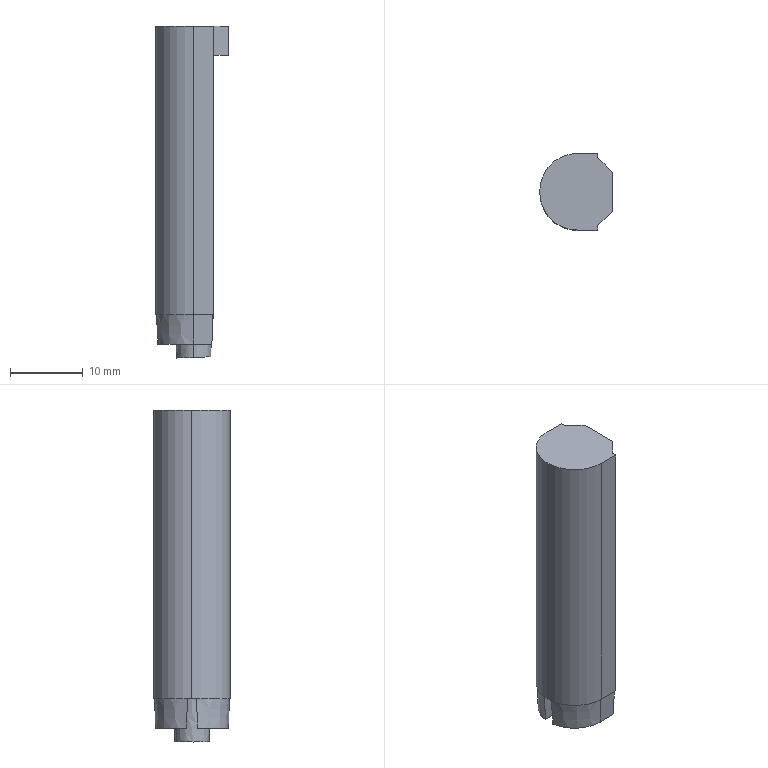Part | Creo | 1 solid | 33 faces | box 10.007 x 10.573 x 45.745 mm | volume 3201 mm3 | plane 24 | cone 4 | spline 3 | cylinder 2 | commonest cylinder face diameters 10.4 x2
STEP:
#1=CARTESIAN_POINT('',(0.,0.,0.));
#2=DIRECTION('',(0.,0.,1.));
#3=DIRECTION('',(1.,0.,0.));
#4=AXIS2_PLACEMENT_3D('',#1,#2,#3);
#5=CARTESIAN_POINT('',(40.585,-87.104,46.111));
#6=VERTEX_POINT('',#5);
#7=CARTESIAN_POINT('',(40.585,-87.104,85.91));
#8=VERTEX_POINT('',#7);
#9=CARTESIAN_POINT('',(40.585,-87.104,46.111));
#10=DIRECTION('',(0.,0.,1.));
#11=VECTOR('',#10,39.799);
#12=LINE('',#9,#11);
#13=EDGE_CURVE('',#6,#8,#12,.T.);
#14=ORIENTED_EDGE('',*,*,#13,.T.);
#15=CARTESIAN_POINT('',(43.392,-87.104,85.91));
#16=VERTEX_POINT('',#15);
#17=CARTESIAN_POINT('',(40.585,-87.104,85.91));
#18=DIRECTION('',(1.,0.,0.));
#19=VECTOR('',#18,2.807);
#20=LINE('',#17,#19);
#21=EDGE_CURVE('',#8,#16,#20,.T.);
#22=ORIENTED_EDGE('',*,*,#21,.T.);
#23=CARTESIAN_POINT('',(43.392,-87.104,46.111));
#24=VERTEX_POINT('',#23);
#25=CARTESIAN_POINT('',(43.392,-87.104,85.91));
#26=DIRECTION('',(0.,0.,-1.));
#27=VECTOR('',#26,39.799);
#28=LINE('',#25,#27);
#29=EDGE_CURVE('',#16,#24,#28,.T.);
#30=ORIENTED_EDGE('',*,*,#29,.T.);
#31=CARTESIAN_POINT('',(43.392,-87.104,46.111));
#32=DIRECTION('',(-1.,0.,0.));
#33=VECTOR('',#32,2.807);
#34=LINE('',#31,#33);
#35=EDGE_CURVE('',#24,#6,#34,.T.);
#36=ORIENTED_EDGE('',*,*,#35,.T.);
#37=EDGE_LOOP('',(#14,#22,#30,#36));
#38=FACE_OUTER_BOUND('',#37,.F.);
#39=CARTESIAN_POINT('',(39.414,-87.104,26.169));
#40=DIRECTION('',(0.,-1.,0.));
#41=DIRECTION('',(0.,0.,-1.));
#42=AXIS2_PLACEMENT_3D('',#39,#40,#41);
#43=PLANE('',#42);
#44=ADVANCED_FACE('',(#38),#43,.T.);
#45=CARTESIAN_POINT('',(35.385,-81.904,85.91));
#46=VERTEX_POINT('',#45);
#47=CARTESIAN_POINT('',(40.585,-81.904,85.91));
#48=DIRECTION('',(0.,0.,1.));
#49=DIRECTION('',(-1.,0.,0.));
#50=AXIS2_PLACEMENT_3D('',#47,#48,#49);
#51=CIRCLE('',#50,5.2);
#52=EDGE_CURVE('',#46,#8,#51,.T.);
#53=ORIENTED_EDGE('',*,*,#52,.T.);
#54=ORIENTED_EDGE('',*,*,#13,.F.);
#55=CARTESIAN_POINT('',(35.385,-81.904,46.111));
#56=VERTEX_POINT('',#55);
#57=CARTESIAN_POINT('',(40.585,-81.904,46.111));
#58=DIRECTION('',(0.,0.,-1.));
#59=DIRECTION('',(0.,-1.,0.));
#60=AXIS2_PLACEMENT_3D('',#57,#58,#59);
#61=CIRCLE('',#60,5.2);
#62=EDGE_CURVE('',#6,#56,#61,.T.);
#63=ORIENTED_EDGE('',*,*,#62,.T.);
#64=CARTESIAN_POINT('',(35.386,-81.817,46.111));
#65=VERTEX_POINT('',#64);
#66=CARTESIAN_POINT('',(40.585,-81.904,46.111));
#67=DIRECTION('',(0.,0.,-1.));
#68=DIRECTION('',(-1.,0.,0.));
#69=AXIS2_PLACEMENT_3D('',#66,#67,#68);
#70=CIRCLE('',#69,5.2);
#71=EDGE_CURVE('',#56,#65,#70,.T.);
#72=ORIENTED_EDGE('',*,*,#71,.T.);
#73=CARTESIAN_POINT('',(35.386,-81.817,85.91));
#74=VERTEX_POINT('',#73);
#75=CARTESIAN_POINT('',(35.386,-81.817,85.91));
#76=DIRECTION('',(0.,0.,-1.));
#77=VECTOR('',#76,39.799);
#78=LINE('',#75,#77);
#79=EDGE_CURVE('',#74,#65,#78,.T.);
#80=ORIENTED_EDGE('',*,*,#79,.F.);
#81=CARTESIAN_POINT('',(40.585,-81.904,85.91));
#82=DIRECTION('',(0.,0.,-1.));
#83=DIRECTION('',(-1.,0.,0.));
#84=AXIS2_PLACEMENT_3D('',#81,#82,#83);
#85=CIRCLE('',#84,5.2);
#86=EDGE_CURVE('',#46,#74,#85,.T.);
#87=ORIENTED_EDGE('',*,*,#86,.F.);
#88=EDGE_LOOP('',(#53,#54,#63,#72,#80,#87));
#89=FACE_OUTER_BOUND('',#88,.F.);
#90=CARTESIAN_POINT('',(40.585,-81.904,26.169));
#91=DIRECTION('',(0.,0.,1.));
#92=DIRECTION('',(1.,0.,0.));
#93=AXIS2_PLACEMENT_3D('',#90,#91,#92);
#94=CYLINDRICAL_SURFACE('',#93,5.2);
#95=ADVANCED_FACE('',(#89),#94,.T.);
#96=CARTESIAN_POINT('',(43.392,-86.504,85.91));
#97=VERTEX_POINT('',#96);
#98=CARTESIAN_POINT('',(43.392,-87.104,85.91));
#99=DIRECTION('',(0.,1.,0.));
#100=VECTOR('',#99,0.6);
#101=LINE('',#98,#100);
#102=EDGE_CURVE('',#16,#97,#101,.T.);
#103=ORIENTED_EDGE('',*,*,#102,.F.);
#104=ORIENTED_EDGE('',*,*,#21,.F.);
#105=ORIENTED_EDGE('',*,*,#52,.F.);
#106=ORIENTED_EDGE('',*,*,#86,.T.);
#107=CARTESIAN_POINT('',(35.385,-81.731,85.91));
#108=VERTEX_POINT('',#107);
#109=CARTESIAN_POINT('',(40.585,-81.731,85.91));
#110=DIRECTION('',(0.,0.,-1.));
#111=DIRECTION('',(-0.9999,-0.01662,0.));
#112=AXIS2_PLACEMENT_3D('',#109,#110,#111);
#113=CIRCLE('',#112,5.2);
#114=EDGE_CURVE('',#74,#108,#113,.T.);
#115=ORIENTED_EDGE('',*,*,#114,.T.);
#116=CARTESIAN_POINT('',(40.585,-76.531,85.91));
#117=VERTEX_POINT('',#116);
#118=CARTESIAN_POINT('',(40.585,-81.731,85.91));
#119=DIRECTION('',(0.,0.,1.));
#120=DIRECTION('',(0.,1.,0.));
#121=AXIS2_PLACEMENT_3D('',#118,#119,#120);
#122=CIRCLE('',#121,5.2);
#123=EDGE_CURVE('',#117,#108,#122,.T.);
#124=ORIENTED_EDGE('',*,*,#123,.F.);
#125=CARTESIAN_POINT('',(43.392,-76.531,85.91));
#126=VERTEX_POINT('',#125);
#127=CARTESIAN_POINT('',(43.392,-76.531,85.91));
#128=DIRECTION('',(-1.,0.,0.));
#129=VECTOR('',#128,2.807);
#130=LINE('',#127,#129);
#131=EDGE_CURVE('',#126,#117,#130,.T.);
#132=ORIENTED_EDGE('',*,*,#131,.F.);
#133=CARTESIAN_POINT('',(43.392,-77.131,85.91));
#134=VERTEX_POINT('',#133);
#135=CARTESIAN_POINT('',(43.392,-77.131,85.91));
#136=DIRECTION('',(0.,1.,0.));
#137=VECTOR('',#136,0.6);
#138=LINE('',#135,#137);
#139=EDGE_CURVE('',#134,#126,#138,.T.);
#140=ORIENTED_EDGE('',*,*,#139,.F.);
#141=CARTESIAN_POINT('',(45.392,-79.131,85.91));
#142=VERTEX_POINT('',#141);
#143=CARTESIAN_POINT('',(45.392,-79.131,85.91));
#144=DIRECTION('',(-0.7071,0.7071,0.));
#145=VECTOR('',#144,2.828);
#146=LINE('',#143,#145);
#147=EDGE_CURVE('',#142,#134,#146,.T.);
#148=ORIENTED_EDGE('',*,*,#147,.F.);
#149=CARTESIAN_POINT('',(45.392,-84.504,85.91));
#150=VERTEX_POINT('',#149);
#151=CARTESIAN_POINT('',(45.392,-84.504,85.91));
#152=DIRECTION('',(0.,1.,0.));
#153=VECTOR('',#152,5.373);
#154=LINE('',#151,#153);
#155=EDGE_CURVE('',#150,#142,#154,.T.);
#156=ORIENTED_EDGE('',*,*,#155,.F.);
#157=CARTESIAN_POINT('',(43.392,-86.504,85.91));
#158=DIRECTION('',(0.7071,0.7071,0.));
#159=VECTOR('',#158,2.828);
#160=LINE('',#157,#159);
#161=EDGE_CURVE('',#97,#150,#160,.T.);
#162=ORIENTED_EDGE('',*,*,#161,.F.);
#163=EDGE_LOOP('',(#103,#104,#105,#106,#115,#124,#132,#140,#148,#156,#162));
#164=FACE_OUTER_BOUND('',#163,.F.);
#165=CARTESIAN_POINT('',(62.144,-0.4125,85.91));
#166=DIRECTION('',(0.,0.,1.));
#167=DIRECTION('',(0.,1.,0.));
#168=AXIS2_PLACEMENT_3D('',#165,#166,#167);
#169=PLANE('',#168);
#170=ADVANCED_FACE('',(#164),#169,.T.);
#171=ORIENTED_EDGE('',*,*,#29,.F.);
#172=ORIENTED_EDGE('',*,*,#102,.T.);
#173=CARTESIAN_POINT('',(43.392,-86.504,81.91));
#174=VERTEX_POINT('',#173);
#175=CARTESIAN_POINT('',(43.392,-86.504,81.91));
#176=DIRECTION('',(0.,0.,1.));
#177=VECTOR('',#176,4.);
#178=LINE('',#175,#177);
#179=EDGE_CURVE('',#174,#97,#178,.T.);
#180=ORIENTED_EDGE('',*,*,#179,.F.);
#181=CARTESIAN_POINT('',(43.392,-77.131,81.91));
#182=VERTEX_POINT('',#181);
#183=CARTESIAN_POINT('',(43.392,-77.131,81.91));
#184=DIRECTION('',(0.,-1.,0.));
#185=VECTOR('',#184,9.373);
#186=LINE('',#183,#185);
#187=EDGE_CURVE('',#182,#174,#186,.T.);
#188=ORIENTED_EDGE('',*,*,#187,.F.);
#189=CARTESIAN_POINT('',(43.392,-77.131,85.91));
#190=DIRECTION('',(0.,0.,-1.));
#191=VECTOR('',#190,4.);
#192=LINE('',#189,#191);
#193=EDGE_CURVE('',#134,#182,#192,.T.);
#194=ORIENTED_EDGE('',*,*,#193,.F.);
#195=ORIENTED_EDGE('',*,*,#139,.T.);
#196=CARTESIAN_POINT('',(43.392,-76.531,46.111));
#197=VERTEX_POINT('',#196);
#198=CARTESIAN_POINT('',(43.392,-76.531,85.91));
#199=DIRECTION('',(0.,0.,-1.));
#200=VECTOR('',#199,39.799);
#201=LINE('',#198,#200);
#202=EDGE_CURVE('',#126,#197,#201,.T.);
#203=ORIENTED_EDGE('',*,*,#202,.T.);
#204=CARTESIAN_POINT('',(43.392,-76.531,46.111));
#205=DIRECTION('',(0.,-1.,0.));
#206=VECTOR('',#205,10.573);
#207=LINE('',#204,#206);
#208=EDGE_CURVE('',#197,#24,#207,.T.);
#209=ORIENTED_EDGE('',*,*,#208,.T.);
#210=EDGE_LOOP('',(#171,#172,#180,#188,#194,#195,#203,#209));
#211=FACE_OUTER_BOUND('',#210,.F.);
#212=CARTESIAN_POINT('',(43.392,-81.817,26.169));
#213=DIRECTION('',(1.,0.,0.));
#214=DIRECTION('',(0.,0.,-1.));
#215=AXIS2_PLACEMENT_3D('',#212,#213,#214);
#216=PLANE('',#215);
#217=ADVANCED_FACE('',(#211),#216,.T.);
#218=CARTESIAN_POINT('',(45.392,-84.504,81.91));
#219=VERTEX_POINT('',#218);
#220=CARTESIAN_POINT('',(45.392,-84.504,81.91));
#221=DIRECTION('',(-0.7071,-0.7071,0.));
#222=VECTOR('',#221,2.828);
#223=LINE('',#220,#222);
#224=EDGE_CURVE('',#219,#174,#223,.T.);
#225=ORIENTED_EDGE('',*,*,#224,.T.);
#226=ORIENTED_EDGE('',*,*,#179,.T.);
#227=ORIENTED_EDGE('',*,*,#161,.T.);
#228=CARTESIAN_POINT('',(45.392,-84.504,81.91));
#229=DIRECTION('',(0.,0.,1.));
#230=VECTOR('',#229,4.);
#231=LINE('',#228,#230);
#232=EDGE_CURVE('',#219,#150,#231,.T.);
#233=ORIENTED_EDGE('',*,*,#232,.F.);
#234=EDGE_LOOP('',(#225,#226,#227,#233));
#235=FACE_OUTER_BOUND('',#234,.F.);
#236=CARTESIAN_POINT('',(43.392,-86.504,81.91));
#237=DIRECTION('',(-0.7071,0.7071,0.));
#238=DIRECTION('',(0.,0.,1.));
#239=AXIS2_PLACEMENT_3D('',#236,#237,#238);
#240=PLANE('',#239);
#241=ADVANCED_FACE('',(#235),#240,.F.);
#242=CARTESIAN_POINT('',(45.392,-79.131,81.91));
#243=VERTEX_POINT('',#242);
#244=CARTESIAN_POINT('',(45.392,-79.131,81.91));
#245=DIRECTION('',(0.,-1.,0.));
#246=VECTOR('',#245,5.373);
#247=LINE('',#244,#246);
#248=EDGE_CURVE('',#243,#219,#247,.T.);
#249=ORIENTED_EDGE('',*,*,#248,.F.);
#250=CARTESIAN_POINT('',(43.392,-77.131,81.91));
#251=DIRECTION('',(0.7071,-0.7071,0.));
#252=VECTOR('',#251,2.828);
#253=LINE('',#250,#252);
#254=EDGE_CURVE('',#182,#243,#253,.T.);
#255=ORIENTED_EDGE('',*,*,#254,.F.);
#256=ORIENTED_EDGE('',*,*,#187,.T.);
#257=ORIENTED_EDGE('',*,*,#224,.F.);
#258=EDGE_LOOP('',(#249,#255,#256,#257));
#259=FACE_OUTER_BOUND('',#258,.F.);
#260=CARTESIAN_POINT('',(43.842,-81.817,81.91));
#261=DIRECTION('',(0.,0.,-1.));
#262=DIRECTION('',(-1.,0.,0.));
#263=AXIS2_PLACEMENT_3D('',#260,#261,#262);
#264=PLANE('',#263);
#265=ADVANCED_FACE('',(#259),#264,.T.);
#266=ORIENTED_EDGE('',*,*,#155,.T.);
#267=CARTESIAN_POINT('',(45.392,-79.131,85.91));
#268=DIRECTION('',(0.,0.,-1.));
#269=VECTOR('',#268,4.);
#270=LINE('',#267,#269);
#271=EDGE_CURVE('',#142,#243,#270,.T.);
#272=ORIENTED_EDGE('',*,*,#271,.T.);
#273=ORIENTED_EDGE('',*,*,#248,.T.);
#274=ORIENTED_EDGE('',*,*,#232,.T.);
#275=EDGE_LOOP('',(#266,#272,#273,#274));
#276=FACE_OUTER_BOUND('',#275,.F.);
#277=CARTESIAN_POINT('',(45.392,-81.817,81.91));
#278=DIRECTION('',(1.,0.,0.));
#279=DIRECTION('',(0.,0.,-1.));
#280=AXIS2_PLACEMENT_3D('',#277,#278,#279);
#281=PLANE('',#280);
#282=ADVANCED_FACE('',(#276),#281,.T.);
#283=ORIENTED_EDGE('',*,*,#254,.T.);
#284=ORIENTED_EDGE('',*,*,#271,.F.);
#285=ORIENTED_EDGE('',*,*,#147,.T.);
#286=ORIENTED_EDGE('',*,*,#193,.T.);
#287=EDGE_LOOP('',(#283,#284,#285,#286));
#288=FACE_OUTER_BOUND('',#287,.F.);
#289=CARTESIAN_POINT('',(45.392,-79.131,81.91));
#290=DIRECTION('',(-0.7071,-0.7071,0.));
#291=DIRECTION('',(0.,0.,1.));
#292=AXIS2_PLACEMENT_3D('',#289,#290,#291);
#293=PLANE('',#292);
#294=ADVANCED_FACE('',(#288),#293,.F.);
#295=ORIENTED_EDGE('',*,*,#202,.F.);
#296=ORIENTED_EDGE('',*,*,#131,.T.);
#297=CARTESIAN_POINT('',(40.585,-76.531,46.111));
#298=VERTEX_POINT('',#297);
#299=CARTESIAN_POINT('',(40.585,-76.531,85.91));
#300=DIRECTION('',(0.,0.,-1.));
#301=VECTOR('',#300,39.799);
#302=LINE('',#299,#301);
#303=EDGE_CURVE('',#117,#298,#302,.T.);
#304=ORIENTED_EDGE('',*,*,#303,.T.);
#305=CARTESIAN_POINT('',(40.585,-76.531,46.111));
#306=DIRECTION('',(1.,0.,0.));
#307=VECTOR('',#306,2.807);
#308=LINE('',#305,#307);
#309=EDGE_CURVE('',#298,#197,#308,.T.);
#310=ORIENTED_EDGE('',*,*,#309,.T.);
#311=EDGE_LOOP('',(#295,#296,#304,#310));
#312=FACE_OUTER_BOUND('',#311,.F.);
#313=CARTESIAN_POINT('',(39.414,-76.531,26.169));
#314=DIRECTION('',(0.,1.,0.));
#315=DIRECTION('',(0.,0.,1.));
#316=AXIS2_PLACEMENT_3D('',#313,#314,#315);
#317=PLANE('',#316);
#318=ADVANCED_FACE('',(#312),#317,.T.);
#319=ORIENTED_EDGE('',*,*,#303,.F.);
#320=ORIENTED_EDGE('',*,*,#123,.T.);
#321=ORIENTED_EDGE('',*,*,#114,.F.);
#322=ORIENTED_EDGE('',*,*,#79,.T.);
#323=CARTESIAN_POINT('',(35.385,-81.731,46.111));
#324=VERTEX_POINT('',#323);
#325=CARTESIAN_POINT('',(40.585,-81.731,46.111));
#326=DIRECTION('',(0.,0.,-1.));
#327=DIRECTION('',(-0.9999,-0.01662,0.));
#328=AXIS2_PLACEMENT_3D('',#325,#326,#327);
#329=CIRCLE('',#328,5.2);
#330=EDGE_CURVE('',#65,#324,#329,.T.);
#331=ORIENTED_EDGE('',*,*,#330,.T.);
#332=CARTESIAN_POINT('',(40.585,-81.731,46.111));
#333=DIRECTION('',(0.,0.,-1.));
#334=DIRECTION('',(-1.,0.,0.));
#335=AXIS2_PLACEMENT_3D('',#332,#333,#334);
#336=CIRCLE('',#335,5.2);
#337=EDGE_CURVE('',#324,#298,#336,.T.);
#338=ORIENTED_EDGE('',*,*,#337,.T.);
#339=EDGE_LOOP('',(#319,#320,#321,#322,#331,#338));
#340=FACE_OUTER_BOUND('',#339,.F.);
#341=CARTESIAN_POINT('',(40.585,-81.731,26.169));
#342=DIRECTION('',(0.,0.,1.));
#343=DIRECTION('',(1.,0.,0.));
#344=AXIS2_PLACEMENT_3D('',#341,#342,#343);
#345=CYLINDRICAL_SURFACE('',#344,5.2);
#346=ADVANCED_FACE('',(#340),#345,.T.);
#347=ORIENTED_EDGE('',*,*,#35,.F.);
#348=ORIENTED_EDGE('',*,*,#208,.F.);
#349=ORIENTED_EDGE('',*,*,#309,.F.);
#350=ORIENTED_EDGE('',*,*,#337,.F.);
#351=ORIENTED_EDGE('',*,*,#330,.F.);
#352=ORIENTED_EDGE('',*,*,#71,.F.);
#353=ORIENTED_EDGE('',*,*,#62,.F.);
#354=EDGE_LOOP('',(#347,#348,#349,#350,#351,#352,#353));
#355=FACE_OUTER_BOUND('',#354,.F.);
#356=CARTESIAN_POINT('',(43.268,-76.661,46.111));
#357=VERTEX_POINT('',#356);
#358=CARTESIAN_POINT('',(40.624,-76.661,46.111));
#359=VERTEX_POINT('',#358);
#360=CARTESIAN_POINT('',(43.268,-76.661,46.111));
#361=DIRECTION('',(-1.,0.,0.));
#362=VECTOR('',#361,2.644);
#363=LINE('',#360,#362);
#364=EDGE_CURVE('',#357,#359,#363,.T.);
#365=ORIENTED_EDGE('',*,*,#364,.F.);
#366=CARTESIAN_POINT('',(43.268,-78.432,46.111));
#367=VERTEX_POINT('',#366);
#368=CARTESIAN_POINT('',(43.268,-78.432,46.111));
#369=DIRECTION('',(0.,1.,0.));
#370=VECTOR('',#369,1.771);
#371=LINE('',#368,#370);
#372=EDGE_CURVE('',#367,#357,#371,.T.);
#373=ORIENTED_EDGE('',*,*,#372,.F.);
#374=CARTESIAN_POINT('',(40.624,-78.432,46.111));
#375=VERTEX_POINT('',#374);
#376=CARTESIAN_POINT('',(40.624,-78.432,46.111));
#377=DIRECTION('',(1.,0.,0.));
#378=VECTOR('',#377,2.644);
#379=LINE('',#376,#378);
#380=EDGE_CURVE('',#375,#367,#379,.T.);
#381=ORIENTED_EDGE('',*,*,#380,.F.);
#382=CARTESIAN_POINT('',(37.296,-81.195,46.111));
#383=VERTEX_POINT('',#382);
#384=CARTESIAN_POINT('',(40.624,-81.817,46.111));
#385=DIRECTION('',(0.,0.,-1.));
#386=DIRECTION('',(-0.983,0.1837,0.));
#387=AXIS2_PLACEMENT_3D('',#384,#385,#386);
#388=CIRCLE('',#387,3.386);
#389=EDGE_CURVE('',#383,#375,#388,.T.);
#390=ORIENTED_EDGE('',*,*,#389,.F.);
#391=CARTESIAN_POINT('',(35.505,-81.195,46.111));
#392=VERTEX_POINT('',#391);
#393=CARTESIAN_POINT('',(37.296,-81.195,46.111));
#394=DIRECTION('',(-1.,0.,0.));
#395=VECTOR('',#394,1.791);
#396=LINE('',#393,#395);
#397=EDGE_CURVE('',#383,#392,#396,.T.);
#398=ORIENTED_EDGE('',*,*,#397,.T.);
#399=CARTESIAN_POINT('',(40.624,-81.817,46.111));
#400=DIRECTION('',(0.,0.,1.));
#401=DIRECTION('',(0.,1.,0.));
#402=AXIS2_PLACEMENT_3D('',#399,#400,#401);
#403=CIRCLE('',#402,5.157);
#404=EDGE_CURVE('',#359,#392,#403,.T.);
#405=ORIENTED_EDGE('',*,*,#404,.F.);
#406=EDGE_LOOP('',(#365,#373,#381,#390,#398,#405));
#407=FACE_BOUND('',#406,.F.);
#408=CARTESIAN_POINT('',(40.625,-84.381,46.111));
#409=VERTEX_POINT('',#408);
#410=CARTESIAN_POINT('',(40.626,-79.254,46.111));
#411=VERTEX_POINT('',#410);
#412=CARTESIAN_POINT('',(40.625,-84.381,46.111));
#413=CARTESIAN_POINT('',(40.443,-84.382,46.111));
#414=CARTESIAN_POINT('',(40.091,-84.345,46.111));
#415=CARTESIAN_POINT('',(39.576,-84.179,46.111));
#416=CARTESIAN_POINT('',(39.107,-83.909,46.111));
#417=CARTESIAN_POINT('',(38.709,-83.552,46.111));
#418=CARTESIAN_POINT('',(38.389,-83.115,46.111));
#419=CARTESIAN_POINT('',(38.168,-82.62,46.111));
#420=CARTESIAN_POINT('',(38.055,-82.091,46.111));
#421=CARTESIAN_POINT('',(38.054,-81.551,46.111));
#422=CARTESIAN_POINT('',(38.166,-81.023,46.111));
#423=CARTESIAN_POINT('',(38.384,-80.529,46.111));
#424=CARTESIAN_POINT('',(38.702,-80.091,46.111));
#425=CARTESIAN_POINT('',(39.1,-79.731,46.111));
#426=CARTESIAN_POINT('',(39.57,-79.458,46.111));
#427=CARTESIAN_POINT('',(40.089,-79.291,46.111));
#428=CARTESIAN_POINT('',(40.442,-79.253,46.111));
#429=CARTESIAN_POINT('',(40.626,-79.254,46.111));
#430=B_SPLINE_CURVE_WITH_KNOTS('',3,(#412,#413,#414,#415,#416,#417,#418,#419,#420,#421,#422,#423,#424,#425,#426,#427,#428,#429),.UNSPECIFIED.,.F.,.F.,(4,1,1,1,1,1,1,1,1,1,1,1,1,1,1,4),(0.,0.06667,0.1333,0.2,0.2667,0.3333,0.4,0.4667,0.5333,0.6,0.6667,0.7333,0.8,0.8667,0.9333,1.),.UNSPECIFIED.);
#431=EDGE_CURVE('',#409,#411,#430,.T.);
#432=ORIENTED_EDGE('',*,*,#431,.T.);
#433=CARTESIAN_POINT('',(41.074,-79.294,46.111));
#434=VERTEX_POINT('',#433);
#435=CARTESIAN_POINT('',(40.626,-79.254,46.111));
#436=CARTESIAN_POINT('',(40.674,-79.254,46.111));
#437=CARTESIAN_POINT('',(40.776,-79.257,46.111));
#438=CARTESIAN_POINT('',(40.926,-79.27,46.111));
#439=CARTESIAN_POINT('',(41.024,-79.285,46.111));
#440=B_SPLINE_CURVE_WITH_KNOTS('',3,(#435,#436,#437,#438,#439,#433),.UNSPECIFIED.,.F.,.F.,(4,1,1,4),(0.,0.3333,0.6667,1.),.UNSPECIFIED.);
#441=EDGE_CURVE('',#411,#434,#440,.T.);
#442=ORIENTED_EDGE('',*,*,#441,.T.);
#443=CARTESIAN_POINT('',(43.303,-79.295,46.111));
#444=VERTEX_POINT('',#443);
#445=CARTESIAN_POINT('',(43.303,-79.295,46.111));
#446=DIRECTION('',(-1.,0.0001161,-0.000004118));
#447=VECTOR('',#446,2.23);
#448=LINE('',#445,#447);
#449=EDGE_CURVE('',#444,#434,#448,.T.);
#450=ORIENTED_EDGE('',*,*,#449,.F.);
#451=CARTESIAN_POINT('',(43.303,-84.34,46.111));
#452=VERTEX_POINT('',#451);
#453=CARTESIAN_POINT('',(43.303,-84.34,46.111));
#454=DIRECTION('',(0.,1.,0.));
#455=VECTOR('',#454,5.046);
#456=LINE('',#453,#455);
#457=EDGE_CURVE('',#452,#444,#456,.T.);
#458=ORIENTED_EDGE('',*,*,#457,.F.);
#459=CARTESIAN_POINT('',(41.071,-84.341,46.111));
#460=VERTEX_POINT('',#459);
#461=CARTESIAN_POINT('',(41.071,-84.341,46.111));
#462=DIRECTION('',(1.,0.0002341,0.000008303));
#463=VECTOR('',#462,2.232);
#464=LINE('',#461,#463);
#465=EDGE_CURVE('',#460,#452,#464,.T.);
#466=ORIENTED_EDGE('',*,*,#465,.F.);
#467=CARTESIAN_POINT('',(40.625,-84.381,46.111));
#468=CARTESIAN_POINT('',(40.674,-84.381,46.111));
#469=CARTESIAN_POINT('',(40.774,-84.378,46.111));
#470=CARTESIAN_POINT('',(40.923,-84.364,46.111));
#471=CARTESIAN_POINT('',(41.022,-84.35,46.111));
#472=CARTESIAN_POINT('',(41.071,-84.341,46.111));
#473=B_SPLINE_CURVE_WITH_KNOTS('',3,(#467,#468,#469,#470,#471,#472),.UNSPECIFIED.,.F.,.F.,(4,1,1,4),(0.,0.3333,0.6667,1.),.UNSPECIFIED.);
#474=EDGE_CURVE('',#409,#460,#473,.T.);
#475=ORIENTED_EDGE('',*,*,#474,.F.);
#476=EDGE_LOOP('',(#432,#442,#450,#458,#466,#475));
#477=FACE_BOUND('',#476,.F.);
#478=CARTESIAN_POINT('',(43.268,-85.203,46.111));
#479=VERTEX_POINT('',#478);
#480=CARTESIAN_POINT('',(40.624,-85.203,46.111));
#481=VERTEX_POINT('',#480);
#482=CARTESIAN_POINT('',(43.268,-85.203,46.111));
#483=DIRECTION('',(-1.,0.,0.));
#484=VECTOR('',#483,2.644);
#485=LINE('',#482,#484);
#486=EDGE_CURVE('',#479,#481,#485,.T.);
#487=ORIENTED_EDGE('',*,*,#486,.F.);
#488=CARTESIAN_POINT('',(43.268,-86.974,46.111));
#489=VERTEX_POINT('',#488);
#490=CARTESIAN_POINT('',(43.268,-86.974,46.111));
#491=DIRECTION('',(0.,1.,0.));
#492=VECTOR('',#491,1.771);
#493=LINE('',#490,#492);
#494=EDGE_CURVE('',#489,#479,#493,.T.);
#495=ORIENTED_EDGE('',*,*,#494,.F.);
#496=CARTESIAN_POINT('',(40.624,-86.974,46.111));
#497=VERTEX_POINT('',#496);
#498=CARTESIAN_POINT('',(40.624,-86.974,46.111));
#499=DIRECTION('',(1.,0.,0.));
#500=VECTOR('',#499,2.644);
#501=LINE('',#498,#500);
#502=EDGE_CURVE('',#497,#489,#501,.T.);
#503=ORIENTED_EDGE('',*,*,#502,.F.);
#504=CARTESIAN_POINT('',(35.505,-82.44,46.111));
#505=VERTEX_POINT('',#504);
#506=CARTESIAN_POINT('',(40.624,-81.817,46.111));
#507=DIRECTION('',(0.,0.,1.));
#508=DIRECTION('',(-0.9927,-0.1206,0.));
#509=AXIS2_PLACEMENT_3D('',#506,#507,#508);
#510=CIRCLE('',#509,5.157);
#511=EDGE_CURVE('',#505,#497,#510,.T.);
#512=ORIENTED_EDGE('',*,*,#511,.F.);
#513=CARTESIAN_POINT('',(37.296,-82.44,46.111));
#514=VERTEX_POINT('',#513);
#515=CARTESIAN_POINT('',(35.505,-82.44,46.111));
#516=DIRECTION('',(1.,0.,0.));
#517=VECTOR('',#516,1.791);
#518=LINE('',#515,#517);
#519=EDGE_CURVE('',#505,#514,#518,.T.);
#520=ORIENTED_EDGE('',*,*,#519,.T.);
#521=CARTESIAN_POINT('',(40.624,-81.817,46.111));
#522=DIRECTION('',(0.,0.,-1.));
#523=DIRECTION('',(0.,-1.,0.));
#524=AXIS2_PLACEMENT_3D('',#521,#522,#523);
#525=CIRCLE('',#524,3.386);
#526=EDGE_CURVE('',#481,#514,#525,.T.);
#527=ORIENTED_EDGE('',*,*,#526,.F.);
#528=EDGE_LOOP('',(#487,#495,#503,#512,#520,#527));
#529=FACE_BOUND('',#528,.F.);
#530=CARTESIAN_POINT('',(17.66,-88.35,46.111));
#531=DIRECTION('',(0.,0.,1.));
#532=DIRECTION('',(-1.,0.,0.));
#533=AXIS2_PLACEMENT_3D('',#530,#531,#532);
#534=PLANE('',#533);
#535=ADVANCED_FACE('',(#355,#407,#477,#529),#534,.F.);
#536=CARTESIAN_POINT('',(43.128,-76.801,42.091));
#537=VERTEX_POINT('',#536);
#538=CARTESIAN_POINT('',(43.268,-76.661,46.111));
#539=DIRECTION('',(-0.03488,-0.03488,-0.9988));
#540=VECTOR('',#539,4.025);
#541=LINE('',#538,#540);
#542=EDGE_CURVE('',#357,#537,#541,.T.);
#543=ORIENTED_EDGE('',*,*,#542,.F.);
#544=ORIENTED_EDGE('',*,*,#364,.T.);
#545=CARTESIAN_POINT('',(40.624,-76.801,42.091));
#546=VERTEX_POINT('',#545);
#547=CARTESIAN_POINT('',(40.624,-76.661,46.111));
#548=DIRECTION('',(0.,-0.0349,-0.9994));
#549=VECTOR('',#548,4.022);
#550=LINE('',#547,#549);
#551=EDGE_CURVE('',#359,#546,#550,.T.);
#552=ORIENTED_EDGE('',*,*,#551,.T.);
#553=CARTESIAN_POINT('',(43.128,-76.801,42.091));
#554=DIRECTION('',(-1.,0.,0.));
#555=VECTOR('',#554,2.504);
#556=LINE('',#553,#555);
#557=EDGE_CURVE('',#537,#546,#556,.T.);
#558=ORIENTED_EDGE('',*,*,#557,.F.);
#559=EDGE_LOOP('',(#543,#544,#552,#558));
#560=FACE_OUTER_BOUND('',#559,.F.);
#561=CARTESIAN_POINT('',(43.137,-76.801,42.091));
#562=DIRECTION('',(0.,0.9994,-0.0349));
#563=DIRECTION('',(0.,0.0349,0.9994));
#564=AXIS2_PLACEMENT_3D('',#561,#562,#563);
#565=PLANE('',#564);
#566=ADVANCED_FACE('',(#560),#565,.T.);
#567=CARTESIAN_POINT('',(43.128,-78.291,42.091));
#568=VERTEX_POINT('',#567);
#569=CARTESIAN_POINT('',(43.268,-78.432,46.111));
#570=DIRECTION('',(-0.03488,0.03488,-0.9988));
#571=VECTOR('',#570,4.025);
#572=LINE('',#569,#571);
#573=EDGE_CURVE('',#367,#568,#572,.T.);
#574=ORIENTED_EDGE('',*,*,#573,.F.);
#575=ORIENTED_EDGE('',*,*,#372,.T.);
#576=ORIENTED_EDGE('',*,*,#542,.T.);
#577=CARTESIAN_POINT('',(43.128,-76.801,42.091));
#578=DIRECTION('',(0.,-1.,0.));
#579=VECTOR('',#578,1.49);
#580=LINE('',#577,#579);
#581=EDGE_CURVE('',#537,#568,#580,.T.);
#582=ORIENTED_EDGE('',*,*,#581,.T.);
#583=EDGE_LOOP('',(#574,#575,#576,#582));
#584=FACE_OUTER_BOUND('',#583,.F.);
#585=CARTESIAN_POINT('',(43.128,-88.35,42.091));
#586=DIRECTION('',(0.9994,0.,-0.0349));
#587=DIRECTION('',(-0.0349,0.,-0.9994));
#588=AXIS2_PLACEMENT_3D('',#585,#586,#587);
#589=PLANE('',#588);
#590=ADVANCED_FACE('',(#584),#589,.T.);
#591=ORIENTED_EDGE('',*,*,#573,.T.);
#592=CARTESIAN_POINT('',(40.624,-78.291,42.091));
#593=VERTEX_POINT('',#592);
#594=CARTESIAN_POINT('',(40.624,-78.291,42.091));
#595=DIRECTION('',(1.,0.,0.));
#596=VECTOR('',#595,2.504);
#597=LINE('',#594,#596);
#598=EDGE_CURVE('',#593,#568,#597,.T.);
#599=ORIENTED_EDGE('',*,*,#598,.F.);
#600=CARTESIAN_POINT('',(40.624,-78.291,42.091));
#601=DIRECTION('',(0.,-0.0349,0.9994));
#602=VECTOR('',#601,4.022);
#603=LINE('',#600,#602);
#604=EDGE_CURVE('',#593,#375,#603,.T.);
#605=ORIENTED_EDGE('',*,*,#604,.T.);
#606=ORIENTED_EDGE('',*,*,#380,.T.);
#607=EDGE_LOOP('',(#591,#599,#605,#606));
#608=FACE_OUTER_BOUND('',#607,.F.);
#609=CARTESIAN_POINT('',(40.624,-78.291,42.091));
#610=DIRECTION('',(0.,-0.9994,-0.0349));
#611=DIRECTION('',(0.,0.0349,-0.9994));
#612=AXIS2_PLACEMENT_3D('',#609,#610,#611);
#613=PLANE('',#612);
#614=ADVANCED_FACE('',(#608),#613,.T.);
#615=ORIENTED_EDGE('',*,*,#581,.F.);
#616=ORIENTED_EDGE('',*,*,#557,.T.);
#617=CARTESIAN_POINT('',(35.666,-81.055,42.091));
#618=VERTEX_POINT('',#617);
#619=CARTESIAN_POINT('',(40.624,-81.817,42.091));
#620=DIRECTION('',(0.,0.,-1.));
#621=DIRECTION('',(-0.9884,0.152,0.));
#622=AXIS2_PLACEMENT_3D('',#619,#620,#621);
#623=CIRCLE('',#622,5.016);
#624=EDGE_CURVE('',#618,#546,#623,.T.);
#625=ORIENTED_EDGE('',*,*,#624,.F.);
#626=CARTESIAN_POINT('',(37.181,-81.055,42.091));
#627=VERTEX_POINT('',#626);
#628=CARTESIAN_POINT('',(37.181,-81.055,42.091));
#629=DIRECTION('',(-1.,0.,0.));
#630=VECTOR('',#629,1.515);
#631=LINE('',#628,#630);
#632=EDGE_CURVE('',#627,#618,#631,.T.);
#633=ORIENTED_EDGE('',*,*,#632,.F.);
#634=CARTESIAN_POINT('',(40.624,-81.817,42.091));
#635=DIRECTION('',(0.,0.,1.));
#636=DIRECTION('',(0.,1.,0.));
#637=AXIS2_PLACEMENT_3D('',#634,#635,#636);
#638=CIRCLE('',#637,3.526);
#639=EDGE_CURVE('',#593,#627,#638,.T.);
#640=ORIENTED_EDGE('',*,*,#639,.F.);
#641=ORIENTED_EDGE('',*,*,#598,.T.);
#642=EDGE_LOOP('',(#615,#616,#625,#633,#640,#641));
#643=FACE_OUTER_BOUND('',#642,.F.);
#644=CARTESIAN_POINT('',(-0.07825,-88.35,42.091));
#645=DIRECTION('',(0.,0.,1.));
#646=DIRECTION('',(0.,1.,0.));
#647=AXIS2_PLACEMENT_3D('',#644,#645,#646);
#648=PLANE('',#647);
#649=ADVANCED_FACE('',(#643),#648,.F.);
#650=ORIENTED_EDGE('',*,*,#551,.F.);
#651=ORIENTED_EDGE('',*,*,#404,.T.);
#652=CARTESIAN_POINT('',(35.666,-81.055,42.091));
#653=CARTESIAN_POINT('',(35.648,-81.071,42.539));
#654=CARTESIAN_POINT('',(35.612,-81.102,43.434));
#655=CARTESIAN_POINT('',(35.558,-81.149,44.774));
#656=CARTESIAN_POINT('',(35.523,-81.18,45.666));
#657=B_SPLINE_CURVE_WITH_KNOTS('',3,(#652,#653,#654,#655,#656,#391),.UNSPECIFIED.,.F.,.F.,(4,1,1,4),(0.,0.3333,0.6667,1.),.UNSPECIFIED.);
#658=EDGE_CURVE('',#618,#392,#657,.T.);
#659=ORIENTED_EDGE('',*,*,#658,.F.);
#660=ORIENTED_EDGE('',*,*,#624,.T.);
#661=EDGE_LOOP('',(#650,#651,#659,#660));
#662=FACE_OUTER_BOUND('',#661,.F.);
#663=CARTESIAN_POINT('',(40.624,-81.817,44.101));
#664=DIRECTION('',(0.,0.,1.));
#665=DIRECTION('',(1.,0.,0.));
#666=AXIS2_PLACEMENT_3D('',#663,#664,#665);
#667=CONICAL_SURFACE('',#666,5.086,2.);
#668=ADVANCED_FACE('',(#662),#667,.T.);
#669=ORIENTED_EDGE('',*,*,#658,.T.);
#670=ORIENTED_EDGE('',*,*,#397,.F.);
#671=CARTESIAN_POINT('',(37.296,-81.195,46.111));
#672=CARTESIAN_POINT('',(37.283,-81.18,45.663));
#673=CARTESIAN_POINT('',(37.257,-81.148,44.769));
#674=CARTESIAN_POINT('',(37.219,-81.102,43.429));
#675=CARTESIAN_POINT('',(37.194,-81.071,42.537));
#676=CARTESIAN_POINT('',(37.181,-81.055,42.091));
#677=B_SPLINE_CURVE_WITH_KNOTS('',3,(#671,#672,#673,#674,#675,#676),.UNSPECIFIED.,.F.,.F.,(4,1,1,4),(0.,0.3333,0.6667,1.),.UNSPECIFIED.);
#678=EDGE_CURVE('',#383,#627,#677,.T.);
#679=ORIENTED_EDGE('',*,*,#678,.T.);
#680=ORIENTED_EDGE('',*,*,#632,.T.);
#681=EDGE_LOOP('',(#669,#670,#679,#680));
#682=FACE_OUTER_BOUND('',#681,.F.);
#683=CARTESIAN_POINT('',(37.188,-81.055,42.091));
#684=DIRECTION('',(0.,-0.9994,-0.0349));
#685=DIRECTION('',(0.,0.0349,-0.9994));
#686=AXIS2_PLACEMENT_3D('',#683,#684,#685);
#687=PLANE('',#686);
#688=ADVANCED_FACE('',(#682),#687,.T.);
#689=ORIENTED_EDGE('',*,*,#604,.F.);
#690=ORIENTED_EDGE('',*,*,#639,.T.);
#691=ORIENTED_EDGE('',*,*,#678,.F.);
#692=ORIENTED_EDGE('',*,*,#389,.T.);
#693=EDGE_LOOP('',(#689,#690,#691,#692));
#694=FACE_OUTER_BOUND('',#693,.F.);
#695=CARTESIAN_POINT('',(40.624,-81.817,44.101));
#696=DIRECTION('',(0.,0.,-1.));
#697=DIRECTION('',(1.,0.,0.));
#698=AXIS2_PLACEMENT_3D('',#695,#696,#697);
#699=CONICAL_SURFACE('',#698,3.456,2.);
#700=ADVANCED_FACE('',(#694),#699,.F.);
#701=CARTESIAN_POINT('',(40.625,-84.177,40.248));
#702=VERTEX_POINT('',#701);
#703=CARTESIAN_POINT('',(40.625,-84.177,40.248));
#704=DIRECTION('',(0.00002655,-0.03491,0.9994));
#705=VECTOR('',#704,5.867);
#706=LINE('',#703,#705);
#707=EDGE_CURVE('',#702,#409,#706,.T.);
#708=ORIENTED_EDGE('',*,*,#707,.F.);
#709=CARTESIAN_POINT('',(40.625,-79.458,40.248));
#710=VERTEX_POINT('',#709);
#711=CARTESIAN_POINT('',(40.468,-79.458,40.242));
#712=CARTESIAN_POINT('',(40.158,-79.493,40.231));
#713=CARTESIAN_POINT('',(39.685,-79.643,40.215));
#714=CARTESIAN_POINT('',(39.247,-79.886,40.2));
#715=CARTESIAN_POINT('',(38.871,-80.213,40.186));
#716=CARTESIAN_POINT('',(38.578,-80.613,40.176));
#717=CARTESIAN_POINT('',(38.374,-81.063,40.169));
#718=CARTESIAN_POINT('',(38.262,-81.558,40.165));
#719=CARTESIAN_POINT('',(38.262,-82.074,40.165));
#720=CARTESIAN_POINT('',(38.373,-82.569,40.169));
#721=CARTESIAN_POINT('',(38.575,-83.018,40.176));
#722=CARTESIAN_POINT('',(38.866,-83.417,40.186));
#723=CARTESIAN_POINT('',(39.241,-83.745,40.199));
#724=CARTESIAN_POINT('',(39.681,-83.99,40.215));
#725=CARTESIAN_POINT('',(40.156,-84.142,40.231));
#726=CARTESIAN_POINT('',(40.467,-84.177,40.242));
#727=CARTESIAN_POINT('',(40.625,-84.177,40.248));
#728=B_SPLINE_CURVE_WITH_KNOTS('',3,(#709,#711,#712,#713,#714,#715,#716,#717,#718,#719,#720,#721,#722,#723,#724,#725,#726,#727),.UNSPECIFIED.,.F.,.F.,(4,1,1,1,1,1,1,1,1,1,1,1,1,1,1,4),(0.,0.06667,0.1333,0.2,0.2667,0.3333,0.4,0.4667,0.5333,0.6,0.6667,0.7333,0.8,0.8667,0.9333,1.),.UNSPECIFIED.);
#729=EDGE_CURVE('',#710,#702,#728,.T.);
#730=ORIENTED_EDGE('',*,*,#729,.F.);
#731=CARTESIAN_POINT('',(40.626,-79.254,46.111));
#732=DIRECTION('',(-0.0001327,-0.0349,-0.9994));
#733=VECTOR('',#732,5.867);
#734=LINE('',#731,#733);
#735=EDGE_CURVE('',#411,#710,#734,.T.);
#736=ORIENTED_EDGE('',*,*,#735,.F.);
#737=ORIENTED_EDGE('',*,*,#431,.F.);
#738=EDGE_LOOP('',(#708,#730,#736,#737));
#739=FACE_OUTER_BOUND('',#738,.F.);
#740=CARTESIAN_POINT('',(40.698,-84.171,40.128));
#741=CARTESIAN_POINT('',(40.702,-84.243,42.189));
#742=CARTESIAN_POINT('',(40.705,-84.315,44.25));
#743=CARTESIAN_POINT('',(40.708,-84.387,46.312));
#744=CARTESIAN_POINT('',(40.674,-84.172,40.127));
#745=CARTESIAN_POINT('',(40.676,-84.244,42.188));
#746=CARTESIAN_POINT('',(40.678,-84.316,44.25));
#747=CARTESIAN_POINT('',(40.68,-84.388,46.311));
#748=CARTESIAN_POINT('',(40.058,-84.183,40.106));
#749=CARTESIAN_POINT('',(40.032,-84.255,42.167));
#750=CARTESIAN_POINT('',(40.005,-84.327,44.228));
#751=CARTESIAN_POINT('',(39.979,-84.4,46.289));
#752=CARTESIAN_POINT('',(38.769,-83.662,40.064));
#753=CARTESIAN_POINT('',(38.717,-83.719,42.125));
#754=CARTESIAN_POINT('',(38.664,-83.775,44.186));
#755=CARTESIAN_POINT('',(38.612,-83.832,46.247));
#756=CARTESIAN_POINT('',(38.022,-81.818,40.038));
#757=CARTESIAN_POINT('',(37.94,-81.818,42.099));
#758=CARTESIAN_POINT('',(37.858,-81.817,44.16));
#759=CARTESIAN_POINT('',(37.776,-81.817,46.221));
#760=CARTESIAN_POINT('',(38.769,-79.973,40.064));
#761=CARTESIAN_POINT('',(38.717,-79.916,42.125));
#762=CARTESIAN_POINT('',(38.664,-79.86,44.186));
#763=CARTESIAN_POINT('',(38.612,-79.803,46.247));
#764=CARTESIAN_POINT('',(40.058,-79.452,40.106));
#765=CARTESIAN_POINT('',(40.032,-79.38,42.167));
#766=CARTESIAN_POINT('',(40.005,-79.308,44.228));
#767=CARTESIAN_POINT('',(39.979,-79.235,46.289));
#768=CARTESIAN_POINT('',(40.673,-79.463,40.127));
#769=CARTESIAN_POINT('',(40.676,-79.391,42.188));
#770=CARTESIAN_POINT('',(40.678,-79.319,44.25));
#771=CARTESIAN_POINT('',(40.68,-79.247,46.311));
#772=CARTESIAN_POINT('',(40.698,-79.464,40.128));
#773=CARTESIAN_POINT('',(40.701,-79.392,42.189));
#774=CARTESIAN_POINT('',(40.705,-79.32,44.25));
#775=CARTESIAN_POINT('',(40.708,-79.248,46.312));
#776=B_SPLINE_SURFACE_WITH_KNOTS('',3,3,((#740,#741,#742,#743),(#744,#745,#746,#747),(#748,#749,#750,#751),(#752,#753,#754,#755),(#756,#757,#758,#759),(#760,#761,#762,#763),(#764,#765,#766,#767),(#768,#769,#770,#771),(#772,#773,#774,#775)),.UNSPECIFIED.,.F.,.F.,.F.,(4,1,1,1,1,1,4),(4,4),(-0.01041,0.,0.25,0.5,0.75,1.,1.01),(-0.01383,1.014),.UNSPECIFIED.);
#777=ADVANCED_FACE('',(#739),#776,.F.);
#778=ORIENTED_EDGE('',*,*,#707,.T.);
#779=ORIENTED_EDGE('',*,*,#474,.T.);
#780=CARTESIAN_POINT('',(41.06,-84.218,42.593));
#781=VERTEX_POINT('',#780);
#782=CARTESIAN_POINT('',(41.06,-84.218,42.593));
#783=CARTESIAN_POINT('',(41.062,-84.232,42.984));
#784=CARTESIAN_POINT('',(41.064,-84.258,43.766));
#785=CARTESIAN_POINT('',(41.068,-84.299,44.939));
#786=CARTESIAN_POINT('',(41.07,-84.327,45.72));
#787=B_SPLINE_CURVE_WITH_KNOTS('',3,(#782,#783,#784,#785,#786,#459),.UNSPECIFIED.,.F.,.F.,(4,1,1,4),(0.,0.3333,0.6667,1.),.UNSPECIFIED.);
#788=EDGE_CURVE('',#781,#460,#787,.T.);
#789=ORIENTED_EDGE('',*,*,#788,.F.);
#790=CARTESIAN_POINT('',(42.949,-81.077,42.593));
#791=VERTEX_POINT('',#790);
#792=CARTESIAN_POINT('',(41.06,-84.218,42.593));
#793=CARTESIAN_POINT('',(41.233,-84.187,42.593));
#794=CARTESIAN_POINT('',(41.561,-84.085,42.594));
#795=CARTESIAN_POINT('',(42.022,-83.837,42.593));
#796=CARTESIAN_POINT('',(42.417,-83.5,42.594));
#797=CARTESIAN_POINT('',(42.73,-83.084,42.593));
#798=CARTESIAN_POINT('',(42.948,-82.61,42.594));
#799=CARTESIAN_POINT('',(43.062,-82.104,42.593));
#800=CARTESIAN_POINT('',(43.068,-81.581,42.594));
#801=CARTESIAN_POINT('',(43.002,-81.244,42.593));
#802=B_SPLINE_CURVE_WITH_KNOTS('',3,(#792,#793,#794,#795,#796,#797,#798,#799,#800,#801,#790),.UNSPECIFIED.,.F.,.F.,(4,1,1,1,1,1,1,1,4),(0.,0.125,0.25,0.375,0.5,0.625,0.75,0.875,1.),.UNSPECIFIED.);
#803=EDGE_CURVE('',#781,#791,#802,.T.);
#804=ORIENTED_EDGE('',*,*,#803,.T.);
#805=CARTESIAN_POINT('',(42.874,-81.101,40.326));
#806=VERTEX_POINT('',#805);
#807=CARTESIAN_POINT('',(42.949,-81.077,42.593));
#808=DIRECTION('',(-0.03326,-0.01058,-0.9994));
#809=VECTOR('',#808,2.269);
#810=LINE('',#807,#809);
#811=EDGE_CURVE('',#791,#806,#810,.T.);
#812=ORIENTED_EDGE('',*,*,#811,.T.);
#813=CARTESIAN_POINT('',(40.625,-84.177,40.248));
#814=CARTESIAN_POINT('',(40.79,-84.177,40.253));
#815=CARTESIAN_POINT('',(41.116,-84.143,40.265));
#816=CARTESIAN_POINT('',(41.589,-83.99,40.281));
#817=CARTESIAN_POINT('',(42.019,-83.743,40.296));
#818=CARTESIAN_POINT('',(42.387,-83.413,40.309));
#819=CARTESIAN_POINT('',(42.678,-83.015,40.319));
#820=CARTESIAN_POINT('',(42.882,-82.563,40.327));
#821=CARTESIAN_POINT('',(42.988,-82.08,40.33));
#822=CARTESIAN_POINT('',(42.99,-81.581,40.33));
#823=CARTESIAN_POINT('',(42.924,-81.26,40.328));
#824=B_SPLINE_CURVE_WITH_KNOTS('',3,(#813,#814,#815,#816,#817,#818,#819,#820,#821,#822,#823,#805),.UNSPECIFIED.,.F.,.F.,(4,1,1,1,1,1,1,1,1,4),(0.,0.1111,0.2222,0.3333,0.4444,0.5556,0.6667,0.7778,0.8889,1.),.UNSPECIFIED.);
#825=EDGE_CURVE('',#702,#806,#824,.T.);
#826=ORIENTED_EDGE('',*,*,#825,.F.);
#827=EDGE_LOOP('',(#778,#779,#789,#804,#812,#826));
#828=FACE_OUTER_BOUND('',#827,.F.);
#829=CARTESIAN_POINT('',(42.841,-81.019,40.205));
#830=CARTESIAN_POINT('',(42.908,-80.995,42.237));
#831=CARTESIAN_POINT('',(42.975,-80.971,44.27));
#832=CARTESIAN_POINT('',(43.042,-80.947,46.303));
#833=CARTESIAN_POINT('',(42.851,-81.046,40.205));
#834=CARTESIAN_POINT('',(42.918,-81.023,42.238));
#835=CARTESIAN_POINT('',(42.985,-81.,44.27));
#836=CARTESIAN_POINT('',(43.052,-80.977,46.303));
#837=CARTESIAN_POINT('',(42.979,-81.424,40.21));
#838=CARTESIAN_POINT('',(43.05,-81.412,42.242));
#839=CARTESIAN_POINT('',(43.121,-81.4,44.275));
#840=CARTESIAN_POINT('',(43.192,-81.388,46.307));
#841=CARTESIAN_POINT('',(43.037,-82.211,40.211));
#842=CARTESIAN_POINT('',(43.11,-82.223,42.244));
#843=CARTESIAN_POINT('',(43.182,-82.234,44.277));
#844=CARTESIAN_POINT('',(43.255,-82.246,46.309));
#845=CARTESIAN_POINT('',(42.598,-83.26,40.197));
#846=CARTESIAN_POINT('',(42.657,-83.304,42.229));
#847=CARTESIAN_POINT('',(42.716,-83.347,44.262));
#848=CARTESIAN_POINT('',(42.776,-83.391,46.295));
#849=CARTESIAN_POINT('',(41.731,-83.997,40.168));
#850=CARTESIAN_POINT('',(41.764,-84.063,42.2));
#851=CARTESIAN_POINT('',(41.797,-84.128,44.233));
#852=CARTESIAN_POINT('',(41.831,-84.194,46.265));
#853=CARTESIAN_POINT('',(40.964,-84.18,40.142));
#854=CARTESIAN_POINT('',(40.974,-84.251,42.174));
#855=CARTESIAN_POINT('',(40.984,-84.322,44.207));
#856=CARTESIAN_POINT('',(40.994,-84.393,46.24));
#857=CARTESIAN_POINT('',(40.565,-84.172,40.128));
#858=CARTESIAN_POINT('',(40.564,-84.243,42.161));
#859=CARTESIAN_POINT('',(40.562,-84.314,44.194));
#860=CARTESIAN_POINT('',(40.56,-84.385,46.226));
#861=CARTESIAN_POINT('',(40.536,-84.171,40.127));
#862=CARTESIAN_POINT('',(40.533,-84.242,42.16));
#863=CARTESIAN_POINT('',(40.531,-84.313,44.193));
#864=CARTESIAN_POINT('',(40.528,-84.384,46.225));
#865=B_SPLINE_SURFACE_WITH_KNOTS('',3,3,((#829,#830,#831,#832),(#833,#834,#835,#836),(#837,#838,#839,#840),(#841,#842,#843,#844),(#845,#846,#847,#848),(#849,#850,#851,#852),(#853,#854,#855,#856),(#857,#858,#859,#860),(#861,#862,#863,#864)),.UNSPECIFIED.,.F.,.F.,.F.,(4,1,1,1,1,1,4),(4,4),(-0.02,0.,0.25,0.5,0.75,1.,1.02),(-0.01383,1.014),.UNSPECIFIED.);
#866=ADVANCED_FACE('',(#828),#865,.F.);
#867=CARTESIAN_POINT('',(43.181,-84.218,42.593));
#868=VERTEX_POINT('',#867);
#869=CARTESIAN_POINT('',(41.06,-84.218,42.593));
#870=DIRECTION('',(1.,0.000245,0.000008697));
#871=VECTOR('',#870,2.12);
#872=LINE('',#869,#871);
#873=EDGE_CURVE('',#781,#868,#872,.T.);
#874=ORIENTED_EDGE('',*,*,#873,.F.);
#875=ORIENTED_EDGE('',*,*,#788,.T.);
#876=ORIENTED_EDGE('',*,*,#465,.T.);
#877=CARTESIAN_POINT('',(43.303,-84.34,46.111));
#878=DIRECTION('',(-0.03488,0.03488,-0.9988));
#879=VECTOR('',#878,3.522);
#880=LINE('',#877,#879);
#881=EDGE_CURVE('',#452,#868,#880,.T.);
#882=ORIENTED_EDGE('',*,*,#881,.T.);
#883=EDGE_LOOP('',(#874,#875,#876,#882));
#884=FACE_OUTER_BOUND('',#883,.F.);
#885=CARTESIAN_POINT('',(40.624,-84.218,42.59));
#886=DIRECTION('',(0.,-0.9994,-0.0349));
#887=DIRECTION('',(0.,0.0349,-0.9994));
#888=AXIS2_PLACEMENT_3D('',#885,#886,#887);
#889=PLANE('',#888);
#890=ADVANCED_FACE('',(#884),#889,.T.);
#891=ORIENTED_EDGE('',*,*,#873,.T.);
#892=CARTESIAN_POINT('',(43.181,-79.417,42.593));
#893=VERTEX_POINT('',#892);
#894=CARTESIAN_POINT('',(43.181,-84.218,42.593));
#895=DIRECTION('',(0.,1.,0.));
#896=VECTOR('',#895,4.8);
#897=LINE('',#894,#896);
#898=EDGE_CURVE('',#868,#893,#897,.T.);
#899=ORIENTED_EDGE('',*,*,#898,.T.);
#900=CARTESIAN_POINT('',(41.063,-79.417,42.593));
#901=VERTEX_POINT('',#900);
#902=CARTESIAN_POINT('',(43.181,-79.417,42.593));
#903=DIRECTION('',(-1.,0.0001268,-0.000004503));
#904=VECTOR('',#903,2.118);
#905=LINE('',#902,#904);
#906=EDGE_CURVE('',#893,#901,#905,.T.);
#907=ORIENTED_EDGE('',*,*,#906,.T.);
#908=CARTESIAN_POINT('',(41.233,-79.449,42.593));
#909=CARTESIAN_POINT('',(41.563,-79.545,42.594));
#910=CARTESIAN_POINT('',(42.04,-79.811,42.593));
#911=CARTESIAN_POINT('',(42.443,-80.172,42.594));
#912=CARTESIAN_POINT('',(42.76,-80.607,42.593));
#913=CARTESIAN_POINT('',(42.898,-80.916,42.593));
#914=CARTESIAN_POINT('',(42.949,-81.077,42.593));
#915=B_SPLINE_CURVE_WITH_KNOTS('',3,(#900,#908,#909,#910,#911,#912,#913,#914),.UNSPECIFIED.,.F.,.F.,(4,1,1,1,1,4),(0.,0.2,0.4,0.6,0.8,1.),.UNSPECIFIED.);
#916=EDGE_CURVE('',#901,#791,#915,.T.);
#917=ORIENTED_EDGE('',*,*,#916,.T.);
#918=ORIENTED_EDGE('',*,*,#803,.F.);
#919=EDGE_LOOP('',(#891,#899,#907,#917,#918));
#920=FACE_OUTER_BOUND('',#919,.F.);
#921=CARTESIAN_POINT('',(-0.07825,-88.35,42.593));
#922=DIRECTION('',(0.,0.,1.));
#923=DIRECTION('',(0.,-1.,0.));
#924=AXIS2_PLACEMENT_3D('',#921,#922,#923);
#925=PLANE('',#924);
#926=ADVANCED_FACE('',(#920),#925,.F.);
#927=CARTESIAN_POINT('',(43.303,-79.295,46.111));
#928=DIRECTION('',(-0.03488,-0.03488,-0.9988));
#929=VECTOR('',#928,3.522);
#930=LINE('',#927,#929);
#931=EDGE_CURVE('',#444,#893,#930,.T.);
#932=ORIENTED_EDGE('',*,*,#931,.T.);
#933=ORIENTED_EDGE('',*,*,#898,.F.);
#934=ORIENTED_EDGE('',*,*,#881,.F.);
#935=ORIENTED_EDGE('',*,*,#457,.T.);
#936=EDGE_LOOP('',(#932,#933,#934,#935));
#937=FACE_OUTER_BOUND('',#936,.F.);
#938=CARTESIAN_POINT('',(43.181,-84.079,42.593));
#939=DIRECTION('',(0.9994,0.,-0.0349));
#940=DIRECTION('',(-0.0349,0.,-0.9994));
#941=AXIS2_PLACEMENT_3D('',#938,#939,#940);
#942=PLANE('',#941);
#943=ADVANCED_FACE('',(#937),#942,.T.);
#944=ORIENTED_EDGE('',*,*,#931,.F.);
#945=ORIENTED_EDGE('',*,*,#449,.T.);
#946=CARTESIAN_POINT('',(41.074,-79.294,46.111));
#947=CARTESIAN_POINT('',(41.072,-79.308,45.72));
#948=CARTESIAN_POINT('',(41.07,-79.336,44.939));
#949=CARTESIAN_POINT('',(41.066,-79.376,43.766));
#950=CARTESIAN_POINT('',(41.064,-79.403,42.984));
#951=CARTESIAN_POINT('',(41.063,-79.417,42.593));
#952=B_SPLINE_CURVE_WITH_KNOTS('',3,(#946,#947,#948,#949,#950,#951),.UNSPECIFIED.,.F.,.F.,(4,1,1,4),(0.,0.3333,0.6667,1.),.UNSPECIFIED.);
#953=EDGE_CURVE('',#434,#901,#952,.T.);
#954=ORIENTED_EDGE('',*,*,#953,.T.);
#955=ORIENTED_EDGE('',*,*,#906,.F.);
#956=EDGE_LOOP('',(#944,#945,#954,#955));
#957=FACE_OUTER_BOUND('',#956,.F.);
#958=CARTESIAN_POINT('',(-0.07825,-79.417,42.59));
#959=DIRECTION('',(0.,0.9994,-0.0349));
#960=DIRECTION('',(0.,0.0349,0.9994));
#961=AXIS2_PLACEMENT_3D('',#958,#959,#960);
#962=PLANE('',#961);
#963=ADVANCED_FACE('',(#957),#962,.T.);
#964=ORIENTED_EDGE('',*,*,#811,.F.);
#965=ORIENTED_EDGE('',*,*,#916,.F.);
#966=ORIENTED_EDGE('',*,*,#953,.F.);
#967=ORIENTED_EDGE('',*,*,#441,.F.);
#968=ORIENTED_EDGE('',*,*,#735,.T.);
#969=CARTESIAN_POINT('',(42.874,-81.101,40.326));
#970=CARTESIAN_POINT('',(42.825,-80.95,40.325));
#971=CARTESIAN_POINT('',(42.697,-80.66,40.32));
#972=CARTESIAN_POINT('',(42.406,-80.254,40.31));
#973=CARTESIAN_POINT('',(42.035,-79.909,40.297));
#974=CARTESIAN_POINT('',(41.596,-79.649,40.282));
#975=CARTESIAN_POINT('',(41.112,-79.491,40.265));
#976=CARTESIAN_POINT('',(40.788,-79.458,40.253));
#977=CARTESIAN_POINT('',(40.625,-79.458,40.248));
#978=B_SPLINE_CURVE_WITH_KNOTS('',3,(#969,#970,#971,#972,#973,#974,#975,#976,#977),.UNSPECIFIED.,.F.,.F.,(4,1,1,1,1,1,4),(0.,0.1667,0.3333,0.5,0.6667,0.8333,1.),.UNSPECIFIED.);
#979=EDGE_CURVE('',#806,#710,#978,.T.);
#980=ORIENTED_EDGE('',*,*,#979,.F.);
#981=EDGE_LOOP('',(#964,#965,#966,#967,#968,#980));
#982=FACE_OUTER_BOUND('',#981,.F.);
#983=CARTESIAN_POINT('',(40.595,-79.463,40.129));
#984=CARTESIAN_POINT('',(40.594,-79.392,42.162));
#985=CARTESIAN_POINT('',(40.593,-79.321,44.195));
#986=CARTESIAN_POINT('',(40.592,-79.25,46.227));
#987=CARTESIAN_POINT('',(40.605,-79.462,40.13));
#988=CARTESIAN_POINT('',(40.604,-79.391,42.162));
#989=CARTESIAN_POINT('',(40.603,-79.32,44.195));
#990=CARTESIAN_POINT('',(40.603,-79.25,46.228));
#991=CARTESIAN_POINT('',(41.123,-79.459,40.147));
#992=CARTESIAN_POINT('',(41.138,-79.388,42.18));
#993=CARTESIAN_POINT('',(41.153,-79.317,44.212));
#994=CARTESIAN_POINT('',(41.168,-79.246,46.245));
#995=CARTESIAN_POINT('',(42.097,-79.789,40.18));
#996=CARTESIAN_POINT('',(42.141,-79.728,42.213));
#997=CARTESIAN_POINT('',(42.186,-79.667,44.245));
#998=CARTESIAN_POINT('',(42.23,-79.607,46.278));
#999=CARTESIAN_POINT('',(42.728,-80.647,40.201));
#1000=CARTESIAN_POINT('',(42.791,-80.612,42.233));
#1001=CARTESIAN_POINT('',(42.855,-80.576,44.266));
#1002=CARTESIAN_POINT('',(42.918,-80.54,46.299));
#1003=CARTESIAN_POINT('',(42.876,-81.121,40.206));
#1004=CARTESIAN_POINT('',(42.943,-81.1,42.239));
#1005=CARTESIAN_POINT('',(43.011,-81.08,44.271));
#1006=CARTESIAN_POINT('',(43.079,-81.059,46.304));
#1007=CARTESIAN_POINT('',(42.878,-81.131,40.206));
#1008=CARTESIAN_POINT('',(42.946,-81.11,42.239));
#1009=CARTESIAN_POINT('',(43.014,-81.09,44.271));
#1010=CARTESIAN_POINT('',(43.082,-81.069,46.304));
#1011=B_SPLINE_SURFACE_WITH_KNOTS('',3,3,((#983,#984,#985,#986),(#987,#988,#989,#990),(#991,#992,#993,#994),(#995,#996,#997,#998),(#999,#1000,#1001,#1002),(#1003,#1004,#1005,#1006),(#1007,#1008,#1009,#1010)),.UNSPECIFIED.,.F.,.F.,.F.,(4,1,1,1,4),(4,4),(-0.00974,0.,0.5,1.,1.01),(-0.01383,1.014),.UNSPECIFIED.);
#1012=ADVANCED_FACE('',(#982),#1011,.F.);
#1013=ORIENTED_EDGE('',*,*,#729,.T.);
#1014=ORIENTED_EDGE('',*,*,#825,.T.);
#1015=ORIENTED_EDGE('',*,*,#979,.T.);
#1016=EDGE_LOOP('',(#1013,#1014,#1015));
#1017=FACE_OUTER_BOUND('',#1016,.F.);
#1018=CARTESIAN_POINT('',(35.85,-81.817,40.081));
#1019=DIRECTION('',(0.0349,0.,-0.9994));
#1020=DIRECTION('',(-0.9994,0.,-0.0349));
#1021=AXIS2_PLACEMENT_3D('',#1018,#1019,#1020);
#1022=PLANE('',#1021);
#1023=ADVANCED_FACE('',(#1017),#1022,.T.);
#1024=CARTESIAN_POINT('',(40.624,-85.344,42.091));
#1025=VERTEX_POINT('',#1024);
#1026=CARTESIAN_POINT('',(40.624,-85.203,46.111));
#1027=DIRECTION('',(0.,-0.0349,-0.9994));
#1028=VECTOR('',#1027,4.022);
#1029=LINE('',#1026,#1028);
#1030=EDGE_CURVE('',#481,#1025,#1029,.T.);
#1031=ORIENTED_EDGE('',*,*,#1030,.T.);
#1032=CARTESIAN_POINT('',(43.128,-85.344,42.091));
#1033=VERTEX_POINT('',#1032);
#1034=CARTESIAN_POINT('',(40.624,-85.344,42.091));
#1035=DIRECTION('',(1.,0.,0.));
#1036=VECTOR('',#1035,2.504);
#1037=LINE('',#1034,#1036);
#1038=EDGE_CURVE('',#1025,#1033,#1037,.T.);
#1039=ORIENTED_EDGE('',*,*,#1038,.T.);
#1040=CARTESIAN_POINT('',(43.268,-85.203,46.111));
#1041=DIRECTION('',(-0.03488,-0.03488,-0.9988));
#1042=VECTOR('',#1041,4.025);
#1043=LINE('',#1040,#1042);
#1044=EDGE_CURVE('',#479,#1033,#1043,.T.);
#1045=ORIENTED_EDGE('',*,*,#1044,.F.);
#1046=ORIENTED_EDGE('',*,*,#486,.T.);
#1047=EDGE_LOOP('',(#1031,#1039,#1045,#1046));
#1048=FACE_OUTER_BOUND('',#1047,.F.);
#1049=CARTESIAN_POINT('',(-0.07825,-85.344,42.091));
#1050=DIRECTION('',(0.,0.9994,-0.0349));
#1051=DIRECTION('',(0.,0.0349,0.9994));
#1052=AXIS2_PLACEMENT_3D('',#1049,#1050,#1051);
#1053=PLANE('',#1052);
#1054=ADVANCED_FACE('',(#1048),#1053,.T.);
#1055=CARTESIAN_POINT('',(37.181,-82.58,42.091));
#1056=VERTEX_POINT('',#1055);
#1057=CARTESIAN_POINT('',(37.181,-82.58,42.091));
#1058=CARTESIAN_POINT('',(37.194,-82.564,42.537));
#1059=CARTESIAN_POINT('',(37.219,-82.533,43.429));
#1060=CARTESIAN_POINT('',(37.257,-82.487,44.769));
#1061=CARTESIAN_POINT('',(37.283,-82.455,45.663));
#1062=B_SPLINE_CURVE_WITH_KNOTS('',3,(#1057,#1058,#1059,#1060,#1061,#513),.UNSPECIFIED.,.F.,.F.,(4,1,1,4),(0.,0.3333,0.6667,1.),.UNSPECIFIED.);
#1063=EDGE_CURVE('',#1056,#514,#1062,.T.);
#1064=ORIENTED_EDGE('',*,*,#1063,.F.);
#1065=CARTESIAN_POINT('',(40.624,-81.817,42.091));
#1066=DIRECTION('',(0.,0.,1.));
#1067=DIRECTION('',(-0.9763,-0.2162,0.));
#1068=AXIS2_PLACEMENT_3D('',#1065,#1066,#1067);
#1069=CIRCLE('',#1068,3.526);
#1070=EDGE_CURVE('',#1056,#1025,#1069,.T.);
#1071=ORIENTED_EDGE('',*,*,#1070,.T.);
#1072=ORIENTED_EDGE('',*,*,#1030,.F.);
#1073=ORIENTED_EDGE('',*,*,#526,.T.);
#1074=EDGE_LOOP('',(#1064,#1071,#1072,#1073));
#1075=FACE_OUTER_BOUND('',#1074,.F.);
#1076=CARTESIAN_POINT('',(40.624,-81.817,44.101));
#1077=DIRECTION('',(0.,0.,-1.));
#1078=DIRECTION('',(1.,0.,0.));
#1079=AXIS2_PLACEMENT_3D('',#1076,#1077,#1078);
#1080=CONICAL_SURFACE('',#1079,3.456,2.);
#1081=ADVANCED_FACE('',(#1075),#1080,.F.);
#1082=ORIENTED_EDGE('',*,*,#1063,.T.);
#1083=ORIENTED_EDGE('',*,*,#519,.F.);
#1084=CARTESIAN_POINT('',(35.666,-82.58,42.091));
#1085=VERTEX_POINT('',#1084);
#1086=CARTESIAN_POINT('',(35.523,-82.455,45.666));
#1087=CARTESIAN_POINT('',(35.558,-82.486,44.774));
#1088=CARTESIAN_POINT('',(35.612,-82.533,43.434));
#1089=CARTESIAN_POINT('',(35.648,-82.564,42.539));
#1090=CARTESIAN_POINT('',(35.666,-82.58,42.091));
#1091=B_SPLINE_CURVE_WITH_KNOTS('',3,(#504,#1086,#1087,#1088,#1089,#1090),.UNSPECIFIED.,.F.,.F.,(4,1,1,4),(0.,0.3333,0.6667,1.),.UNSPECIFIED.);
#1092=EDGE_CURVE('',#505,#1085,#1091,.T.);
#1093=ORIENTED_EDGE('',*,*,#1092,.T.);
#1094=CARTESIAN_POINT('',(35.666,-82.58,42.091));
#1095=DIRECTION('',(1.,0.,0.));
#1096=VECTOR('',#1095,1.515);
#1097=LINE('',#1094,#1096);
#1098=EDGE_CURVE('',#1085,#1056,#1097,.T.);
#1099=ORIENTED_EDGE('',*,*,#1098,.T.);
#1100=EDGE_LOOP('',(#1082,#1083,#1093,#1099));
#1101=FACE_OUTER_BOUND('',#1100,.F.);
#1102=CARTESIAN_POINT('',(35.656,-82.58,42.091));
#1103=DIRECTION('',(0.,0.9994,-0.0349));
#1104=DIRECTION('',(0.,0.0349,0.9994));
#1105=AXIS2_PLACEMENT_3D('',#1102,#1103,#1104);
#1106=PLANE('',#1105);
#1107=ADVANCED_FACE('',(#1101),#1106,.T.);
#1108=ORIENTED_EDGE('',*,*,#1092,.F.);
#1109=ORIENTED_EDGE('',*,*,#511,.T.);
#1110=CARTESIAN_POINT('',(40.624,-86.834,42.091));
#1111=VERTEX_POINT('',#1110);
#1112=CARTESIAN_POINT('',(40.624,-86.834,42.091));
#1113=DIRECTION('',(0.,-0.0349,0.9994));
#1114=VECTOR('',#1113,4.022);
#1115=LINE('',#1112,#1114);
#1116=EDGE_CURVE('',#1111,#497,#1115,.T.);
#1117=ORIENTED_EDGE('',*,*,#1116,.F.);
#1118=CARTESIAN_POINT('',(40.624,-81.817,42.091));
#1119=DIRECTION('',(0.,0.,-1.));
#1120=DIRECTION('',(0.,-1.,0.));
#1121=AXIS2_PLACEMENT_3D('',#1118,#1119,#1120);
#1122=CIRCLE('',#1121,5.016);
#1123=EDGE_CURVE('',#1111,#1085,#1122,.T.);
#1124=ORIENTED_EDGE('',*,*,#1123,.T.);
#1125=EDGE_LOOP('',(#1108,#1109,#1117,#1124));
#1126=FACE_OUTER_BOUND('',#1125,.F.);
#1127=CARTESIAN_POINT('',(40.624,-81.817,44.101));
#1128=DIRECTION('',(0.,0.,1.));
#1129=DIRECTION('',(1.,0.,0.));
#1130=AXIS2_PLACEMENT_3D('',#1127,#1128,#1129);
#1131=CONICAL_SURFACE('',#1130,5.086,2.);
#1132=ADVANCED_FACE('',(#1126),#1131,.T.);
#1133=ORIENTED_EDGE('',*,*,#1116,.T.);
#1134=ORIENTED_EDGE('',*,*,#502,.T.);
#1135=CARTESIAN_POINT('',(43.128,-86.834,42.091));
#1136=VERTEX_POINT('',#1135);
#1137=CARTESIAN_POINT('',(43.268,-86.974,46.111));
#1138=DIRECTION('',(-0.03488,0.03488,-0.9988));
#1139=VECTOR('',#1138,4.025);
#1140=LINE('',#1137,#1139);
#1141=EDGE_CURVE('',#489,#1136,#1140,.T.);
#1142=ORIENTED_EDGE('',*,*,#1141,.T.);
#1143=CARTESIAN_POINT('',(43.128,-86.834,42.091));
#1144=DIRECTION('',(-1.,0.,0.));
#1145=VECTOR('',#1144,2.504);
#1146=LINE('',#1143,#1145);
#1147=EDGE_CURVE('',#1136,#1111,#1146,.T.);
#1148=ORIENTED_EDGE('',*,*,#1147,.T.);
#1149=EDGE_LOOP('',(#1133,#1134,#1142,#1148));
#1150=FACE_OUTER_BOUND('',#1149,.F.);
#1151=CARTESIAN_POINT('',(-0.07825,-86.834,42.091));
#1152=DIRECTION('',(0.,-0.9994,-0.0349));
#1153=DIRECTION('',(0.,0.0349,-0.9994));
#1154=AXIS2_PLACEMENT_3D('',#1151,#1152,#1153);
#1155=PLANE('',#1154);
#1156=ADVANCED_FACE('',(#1150),#1155,.T.);
#1157=ORIENTED_EDGE('',*,*,#1141,.F.);
#1158=ORIENTED_EDGE('',*,*,#494,.T.);
#1159=ORIENTED_EDGE('',*,*,#1044,.T.);
#1160=CARTESIAN_POINT('',(43.128,-85.344,42.091));
#1161=DIRECTION('',(0.,-1.,0.));
#1162=VECTOR('',#1161,1.49);
#1163=LINE('',#1160,#1162);
#1164=EDGE_CURVE('',#1033,#1136,#1163,.T.);
#1165=ORIENTED_EDGE('',*,*,#1164,.T.);
#1166=EDGE_LOOP('',(#1157,#1158,#1159,#1165));
#1167=FACE_OUTER_BOUND('',#1166,.F.);
#1168=CARTESIAN_POINT('',(43.128,-88.35,42.091));
#1169=DIRECTION('',(0.9994,0.,-0.0349));
#1170=DIRECTION('',(-0.0349,0.,-0.9994));
#1171=AXIS2_PLACEMENT_3D('',#1168,#1169,#1170);
#1172=PLANE('',#1171);
#1173=ADVANCED_FACE('',(#1167),#1172,.T.);
#1174=ORIENTED_EDGE('',*,*,#1164,.F.);
#1175=ORIENTED_EDGE('',*,*,#1038,.F.);
#1176=ORIENTED_EDGE('',*,*,#1070,.F.);
#1177=ORIENTED_EDGE('',*,*,#1098,.F.);
#1178=ORIENTED_EDGE('',*,*,#1123,.F.);
#1179=ORIENTED_EDGE('',*,*,#1147,.F.);
#1180=EDGE_LOOP('',(#1174,#1175,#1176,#1177,#1178,#1179));
#1181=FACE_OUTER_BOUND('',#1180,.F.);
#1182=CARTESIAN_POINT('',(-0.07825,-88.35,42.091));
#1183=DIRECTION('',(0.,0.,1.));
#1184=DIRECTION('',(0.,1.,0.));
#1185=AXIS2_PLACEMENT_3D('',#1182,#1183,#1184);
#1186=PLANE('',#1185);
#1187=ADVANCED_FACE('',(#1181),#1186,.F.);
#1188=CLOSED_SHELL('',(#44,#95,#170,#217,#241,#265,#282,#294,#318,#346,#535,#566,#590,#614,#649,#668,#688,#700,#777,#866,#890,#926,#943,#963,#1012,#1023,#1054,#1081,#1107,#1132,#1156,#1173,#1187));
#1189=MANIFOLD_SOLID_BREP('',#1188);
#1190=(LENGTH_UNIT()NAMED_UNIT(*)SI_UNIT(.MILLI.,.METRE.));
#1191=UNCERTAINTY_MEASURE_WITH_UNIT(LENGTH_MEASURE(0.004805),#1190,'','');
#1192=(NAMED_UNIT(*)PLANE_ANGLE_UNIT()SI_UNIT($,.RADIAN.));
#1193=PLANE_ANGLE_MEASURE_WITH_UNIT(PLANE_ANGLE_MEASURE(0.01745),#1192);
#1194=(CONVERSION_BASED_UNIT('DEGREE',#1193)NAMED_UNIT(*)PLANE_ANGLE_UNIT());
#1195=(NAMED_UNIT(*)SI_UNIT($,.STERADIAN.)SOLID_ANGLE_UNIT());
#1196=(GEOMETRIC_REPRESENTATION_CONTEXT(3)GLOBAL_UNCERTAINTY_ASSIGNED_CONTEXT((#1191))GLOBAL_UNIT_ASSIGNED_CONTEXT((#1190,#1194,#1195))REPRESENTATION_CONTEXT('',''));
#1197=ADVANCED_BREP_SHAPE_REPRESENTATION('',(#4,#1189),#1196);